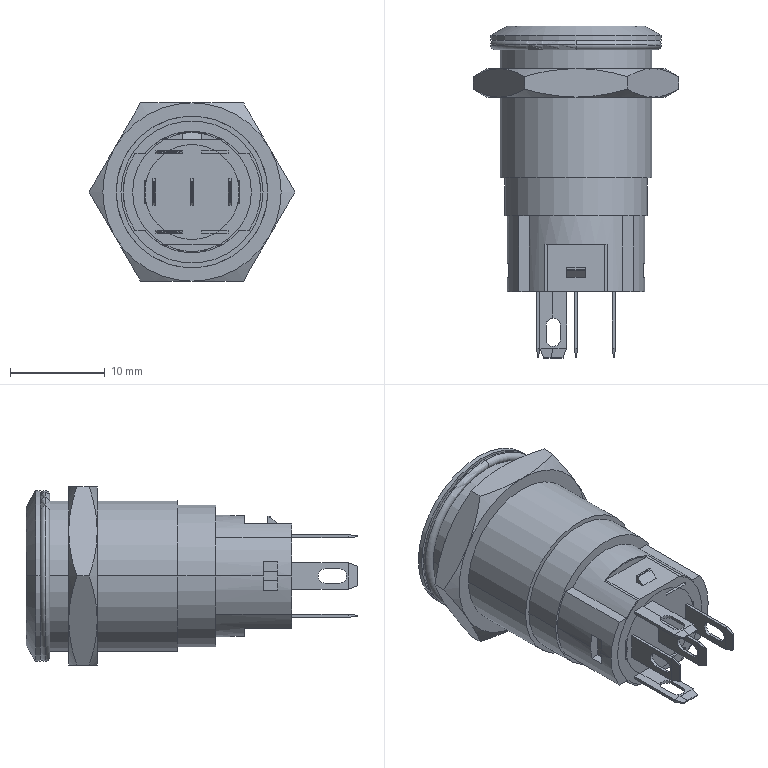Part | NX | features BREP 6 | 6 solids | 223 faces | box 21.708 x 35 x 18.8 mm | volume 5416 mm3 | plane 164 | cylinder 41 | cone 14 | torus 4 | commonest cylinder face diameters 1.5 x14 10 x8 12.536 x6 16 x4 14.5 x3 12.8 x2